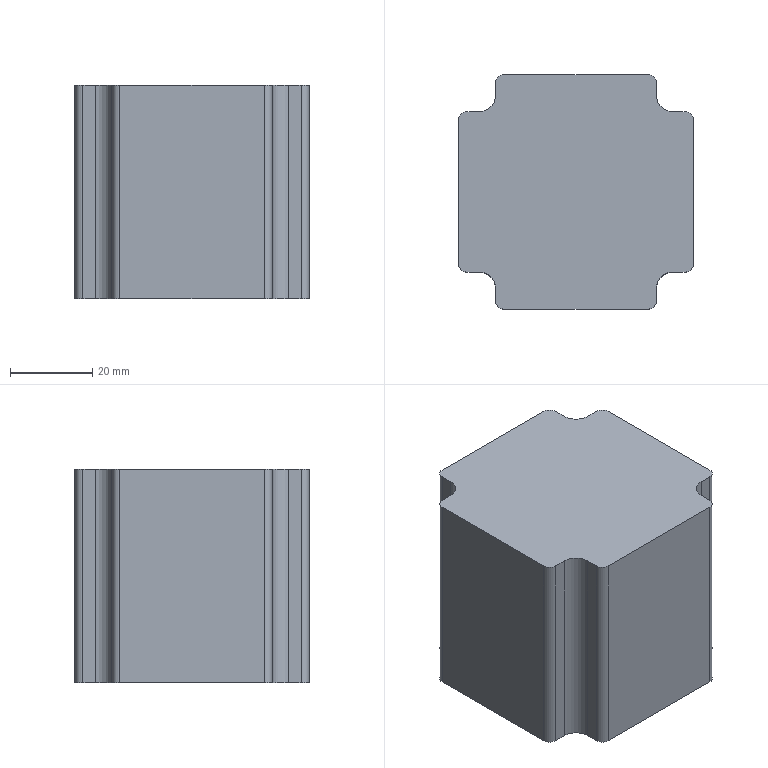Part | SolidWorks | features BaseBody 1 | 1 solid | 26 faces | box 57 x 57 x 52 mm | volume 152457 mm3 | plane 14 | cylinder 12 | commonest cylinder face diameters 4 x8 8 x4
STEP:
#1=CARTESIAN_POINT('',(19.5,26.5,0.));
#2=VERTEX_POINT('',#1);
#3=CARTESIAN_POINT('',(17.5,28.5,0.));
#4=VERTEX_POINT('',#3);
#5=CARTESIAN_POINT('',(17.5,26.5,0.));
#6=DIRECTION('',(0.,0.,1.));
#7=DIRECTION('',(-1.,0.,0.));
#8=AXIS2_PLACEMENT_3D('',#5,#6,#7);
#9=CIRCLE('',#8,2.);
#10=EDGE_CURVE('',#2,#4,#9,.T.);
#11=ORIENTED_EDGE('',*,*,#10,.F.);
#12=CARTESIAN_POINT('',(19.5,23.5,0.));
#13=VERTEX_POINT('',#12);
#14=CARTESIAN_POINT('',(19.5,26.5,0.));
#15=DIRECTION('',(0.,1.,0.));
#16=VECTOR('',#15,1000.);
#17=LINE('',#14,#16);
#18=EDGE_CURVE('',#13,#2,#17,.T.);
#19=ORIENTED_EDGE('',*,*,#18,.F.);
#20=CARTESIAN_POINT('',(23.5,19.5,0.));
#21=VERTEX_POINT('',#20);
#22=CARTESIAN_POINT('',(23.5,23.5,0.));
#23=DIRECTION('',(0.,0.,-1.));
#24=DIRECTION('',(1.,0.,0.));
#25=AXIS2_PLACEMENT_3D('',#22,#23,#24);
#26=CIRCLE('',#25,4.);
#27=EDGE_CURVE('',#21,#13,#26,.T.);
#28=ORIENTED_EDGE('',*,*,#27,.F.);
#29=CARTESIAN_POINT('',(26.5,19.5,0.));
#30=VERTEX_POINT('',#29);
#31=CARTESIAN_POINT('',(23.5,19.5,0.));
#32=DIRECTION('',(-1.,0.,0.));
#33=VECTOR('',#32,1000.);
#34=LINE('',#31,#33);
#35=EDGE_CURVE('',#30,#21,#34,.T.);
#36=ORIENTED_EDGE('',*,*,#35,.F.);
#37=CARTESIAN_POINT('',(28.5,17.5,0.));
#38=VERTEX_POINT('',#37);
#39=CARTESIAN_POINT('',(26.5,17.5,0.));
#40=DIRECTION('',(0.,0.,1.));
#41=DIRECTION('',(-1.,0.,0.));
#42=AXIS2_PLACEMENT_3D('',#39,#40,#41);
#43=CIRCLE('',#42,2.);
#44=EDGE_CURVE('',#38,#30,#43,.T.);
#45=ORIENTED_EDGE('',*,*,#44,.F.);
#46=CARTESIAN_POINT('',(28.5,-17.5,0.));
#47=VERTEX_POINT('',#46);
#48=CARTESIAN_POINT('',(28.5,17.5,0.));
#49=DIRECTION('',(0.,1.,0.));
#50=VECTOR('',#49,1000.);
#51=LINE('',#48,#50);
#52=EDGE_CURVE('',#47,#38,#51,.T.);
#53=ORIENTED_EDGE('',*,*,#52,.F.);
#54=CARTESIAN_POINT('',(26.5,-19.5,0.));
#55=VERTEX_POINT('',#54);
#56=CARTESIAN_POINT('',(26.5,-17.5,0.));
#57=DIRECTION('',(0.,0.,1.));
#58=DIRECTION('',(-1.,0.,0.));
#59=AXIS2_PLACEMENT_3D('',#56,#57,#58);
#60=CIRCLE('',#59,2.);
#61=EDGE_CURVE('',#55,#47,#60,.T.);
#62=ORIENTED_EDGE('',*,*,#61,.F.);
#63=CARTESIAN_POINT('',(23.5,-19.5,0.));
#64=VERTEX_POINT('',#63);
#65=CARTESIAN_POINT('',(26.5,-19.5,0.));
#66=DIRECTION('',(1.,0.,0.));
#67=VECTOR('',#66,1000.);
#68=LINE('',#65,#67);
#69=EDGE_CURVE('',#64,#55,#68,.T.);
#70=ORIENTED_EDGE('',*,*,#69,.F.);
#71=CARTESIAN_POINT('',(19.5,-23.5,0.));
#72=VERTEX_POINT('',#71);
#73=CARTESIAN_POINT('',(23.5,-23.5,0.));
#74=DIRECTION('',(0.,0.,-1.));
#75=DIRECTION('',(-1.,0.,0.));
#76=AXIS2_PLACEMENT_3D('',#73,#74,#75);
#77=CIRCLE('',#76,4.);
#78=EDGE_CURVE('',#72,#64,#77,.T.);
#79=ORIENTED_EDGE('',*,*,#78,.F.);
#80=CARTESIAN_POINT('',(19.5,-26.5,0.));
#81=VERTEX_POINT('',#80);
#82=CARTESIAN_POINT('',(19.5,-23.5,0.));
#83=DIRECTION('',(0.,1.,0.));
#84=VECTOR('',#83,1000.);
#85=LINE('',#82,#84);
#86=EDGE_CURVE('',#81,#72,#85,.T.);
#87=ORIENTED_EDGE('',*,*,#86,.F.);
#88=CARTESIAN_POINT('',(17.5,-28.5,0.));
#89=VERTEX_POINT('',#88);
#90=CARTESIAN_POINT('',(17.5,-26.5,0.));
#91=DIRECTION('',(0.,0.,1.));
#92=DIRECTION('',(-1.,0.,0.));
#93=AXIS2_PLACEMENT_3D('',#90,#91,#92);
#94=CIRCLE('',#93,2.);
#95=EDGE_CURVE('',#89,#81,#94,.T.);
#96=ORIENTED_EDGE('',*,*,#95,.F.);
#97=CARTESIAN_POINT('',(-17.5,-28.5,0.));
#98=VERTEX_POINT('',#97);
#99=CARTESIAN_POINT('',(17.5,-28.5,0.));
#100=DIRECTION('',(1.,0.,0.));
#101=VECTOR('',#100,1000.);
#102=LINE('',#99,#101);
#103=EDGE_CURVE('',#98,#89,#102,.T.);
#104=ORIENTED_EDGE('',*,*,#103,.F.);
#105=CARTESIAN_POINT('',(-19.5,-26.5,0.));
#106=VERTEX_POINT('',#105);
#107=CARTESIAN_POINT('',(-17.5,-26.5,0.));
#108=DIRECTION('',(0.,0.,1.));
#109=DIRECTION('',(-1.,0.,0.));
#110=AXIS2_PLACEMENT_3D('',#107,#108,#109);
#111=CIRCLE('',#110,2.);
#112=EDGE_CURVE('',#106,#98,#111,.T.);
#113=ORIENTED_EDGE('',*,*,#112,.F.);
#114=CARTESIAN_POINT('',(-19.5,-23.5,0.));
#115=VERTEX_POINT('',#114);
#116=CARTESIAN_POINT('',(-19.5,-26.5,0.));
#117=DIRECTION('',(0.,-1.,0.));
#118=VECTOR('',#117,1000.);
#119=LINE('',#116,#118);
#120=EDGE_CURVE('',#115,#106,#119,.T.);
#121=ORIENTED_EDGE('',*,*,#120,.F.);
#122=CARTESIAN_POINT('',(-23.5,-19.5,0.));
#123=VERTEX_POINT('',#122);
#124=CARTESIAN_POINT('',(-23.5,-23.5,0.));
#125=DIRECTION('',(0.,0.,-1.));
#126=DIRECTION('',(1.,0.,0.));
#127=AXIS2_PLACEMENT_3D('',#124,#125,#126);
#128=CIRCLE('',#127,4.);
#129=EDGE_CURVE('',#123,#115,#128,.T.);
#130=ORIENTED_EDGE('',*,*,#129,.F.);
#131=CARTESIAN_POINT('',(-26.5,-19.5,0.));
#132=VERTEX_POINT('',#131);
#133=CARTESIAN_POINT('',(-23.5,-19.5,0.));
#134=DIRECTION('',(1.,0.,0.));
#135=VECTOR('',#134,1000.);
#136=LINE('',#133,#135);
#137=EDGE_CURVE('',#132,#123,#136,.T.);
#138=ORIENTED_EDGE('',*,*,#137,.F.);
#139=CARTESIAN_POINT('',(-28.5,-17.5,0.));
#140=VERTEX_POINT('',#139);
#141=CARTESIAN_POINT('',(-26.5,-17.5,0.));
#142=DIRECTION('',(0.,0.,1.));
#143=DIRECTION('',(-1.,0.,0.));
#144=AXIS2_PLACEMENT_3D('',#141,#142,#143);
#145=CIRCLE('',#144,2.);
#146=EDGE_CURVE('',#140,#132,#145,.T.);
#147=ORIENTED_EDGE('',*,*,#146,.F.);
#148=CARTESIAN_POINT('',(-28.5,17.5,0.));
#149=VERTEX_POINT('',#148);
#150=CARTESIAN_POINT('',(-28.5,-17.5,0.));
#151=DIRECTION('',(0.,-1.,0.));
#152=VECTOR('',#151,1000.);
#153=LINE('',#150,#152);
#154=EDGE_CURVE('',#149,#140,#153,.T.);
#155=ORIENTED_EDGE('',*,*,#154,.F.);
#156=CARTESIAN_POINT('',(-26.5,19.5,0.));
#157=VERTEX_POINT('',#156);
#158=CARTESIAN_POINT('',(-26.5,17.5,0.));
#159=DIRECTION('',(0.,0.,1.));
#160=DIRECTION('',(-1.,0.,0.));
#161=AXIS2_PLACEMENT_3D('',#158,#159,#160);
#162=CIRCLE('',#161,2.);
#163=EDGE_CURVE('',#157,#149,#162,.T.);
#164=ORIENTED_EDGE('',*,*,#163,.F.);
#165=CARTESIAN_POINT('',(-23.5,19.5,0.));
#166=VERTEX_POINT('',#165);
#167=CARTESIAN_POINT('',(-26.5,19.5,0.));
#168=DIRECTION('',(-1.,0.,0.));
#169=VECTOR('',#168,1000.);
#170=LINE('',#167,#169);
#171=EDGE_CURVE('',#166,#157,#170,.T.);
#172=ORIENTED_EDGE('',*,*,#171,.F.);
#173=CARTESIAN_POINT('',(-19.5,23.5,0.));
#174=VERTEX_POINT('',#173);
#175=CARTESIAN_POINT('',(-23.5,23.5,0.));
#176=DIRECTION('',(0.,0.,-1.));
#177=DIRECTION('',(1.,0.,0.));
#178=AXIS2_PLACEMENT_3D('',#175,#176,#177);
#179=CIRCLE('',#178,4.);
#180=EDGE_CURVE('',#174,#166,#179,.T.);
#181=ORIENTED_EDGE('',*,*,#180,.F.);
#182=CARTESIAN_POINT('',(-19.5,26.5,0.));
#183=VERTEX_POINT('',#182);
#184=CARTESIAN_POINT('',(-19.5,23.5,0.));
#185=DIRECTION('',(0.,-1.,0.));
#186=VECTOR('',#185,1000.);
#187=LINE('',#184,#186);
#188=EDGE_CURVE('',#183,#174,#187,.T.);
#189=ORIENTED_EDGE('',*,*,#188,.F.);
#190=CARTESIAN_POINT('',(-17.5,28.5,0.));
#191=VERTEX_POINT('',#190);
#192=CARTESIAN_POINT('',(-17.5,26.5,0.));
#193=DIRECTION('',(0.,0.,1.));
#194=DIRECTION('',(-1.,0.,0.));
#195=AXIS2_PLACEMENT_3D('',#192,#193,#194);
#196=CIRCLE('',#195,2.);
#197=EDGE_CURVE('',#191,#183,#196,.T.);
#198=ORIENTED_EDGE('',*,*,#197,.F.);
#199=CARTESIAN_POINT('',(-17.5,28.5,0.));
#200=DIRECTION('',(-1.,0.,0.));
#201=VECTOR('',#200,1000.);
#202=LINE('',#199,#201);
#203=EDGE_CURVE('',#4,#191,#202,.T.);
#204=ORIENTED_EDGE('',*,*,#203,.F.);
#205=EDGE_LOOP('',(#11,#19,#28,#36,#45,#53,#62,#70,#79,#87,#96,#104,#113,#121,#130,#138,#147,#155,#164,#172,#181,#189,#198,#204));
#206=FACE_OUTER_BOUND('',#205,.T.);
#207=CARTESIAN_POINT('',(17.5,26.5,0.));
#208=DIRECTION('',(0.,0.,-1.));
#209=DIRECTION('',(0.,-1.,0.));
#210=AXIS2_PLACEMENT_3D('',#207,#208,#209);
#211=PLANE('',#210);
#212=ADVANCED_FACE('',(#206),#211,.T.);
#213=CARTESIAN_POINT('',(19.5,26.5,52.));
#214=VERTEX_POINT('',#213);
#215=CARTESIAN_POINT('',(17.5,28.5,52.));
#216=VERTEX_POINT('',#215);
#217=CARTESIAN_POINT('',(17.5,26.5,52.));
#218=DIRECTION('',(0.,0.,1.));
#219=DIRECTION('',(-1.,0.,0.));
#220=AXIS2_PLACEMENT_3D('',#217,#218,#219);
#221=CIRCLE('',#220,2.);
#222=EDGE_CURVE('',#214,#216,#221,.T.);
#223=ORIENTED_EDGE('',*,*,#222,.T.);
#224=CARTESIAN_POINT('',(-17.5,28.5,52.));
#225=VERTEX_POINT('',#224);
#226=CARTESIAN_POINT('',(-17.5,28.5,52.));
#227=DIRECTION('',(-1.,0.,0.));
#228=VECTOR('',#227,1000.);
#229=LINE('',#226,#228);
#230=EDGE_CURVE('',#216,#225,#229,.T.);
#231=ORIENTED_EDGE('',*,*,#230,.T.);
#232=CARTESIAN_POINT('',(-19.5,26.5,52.));
#233=VERTEX_POINT('',#232);
#234=CARTESIAN_POINT('',(-17.5,26.5,52.));
#235=DIRECTION('',(0.,0.,1.));
#236=DIRECTION('',(-1.,0.,0.));
#237=AXIS2_PLACEMENT_3D('',#234,#235,#236);
#238=CIRCLE('',#237,2.);
#239=EDGE_CURVE('',#225,#233,#238,.T.);
#240=ORIENTED_EDGE('',*,*,#239,.T.);
#241=CARTESIAN_POINT('',(-19.5,23.5,52.));
#242=VERTEX_POINT('',#241);
#243=CARTESIAN_POINT('',(-19.5,23.5,52.));
#244=DIRECTION('',(0.,-1.,0.));
#245=VECTOR('',#244,1000.);
#246=LINE('',#243,#245);
#247=EDGE_CURVE('',#233,#242,#246,.T.);
#248=ORIENTED_EDGE('',*,*,#247,.T.);
#249=CARTESIAN_POINT('',(-23.5,19.5,52.));
#250=VERTEX_POINT('',#249);
#251=CARTESIAN_POINT('',(-23.5,23.5,52.));
#252=DIRECTION('',(0.,0.,-1.));
#253=DIRECTION('',(1.,0.,0.));
#254=AXIS2_PLACEMENT_3D('',#251,#252,#253);
#255=CIRCLE('',#254,4.);
#256=EDGE_CURVE('',#242,#250,#255,.T.);
#257=ORIENTED_EDGE('',*,*,#256,.T.);
#258=CARTESIAN_POINT('',(-26.5,19.5,52.));
#259=VERTEX_POINT('',#258);
#260=CARTESIAN_POINT('',(-26.5,19.5,52.));
#261=DIRECTION('',(-1.,0.,0.));
#262=VECTOR('',#261,1000.);
#263=LINE('',#260,#262);
#264=EDGE_CURVE('',#250,#259,#263,.T.);
#265=ORIENTED_EDGE('',*,*,#264,.T.);
#266=CARTESIAN_POINT('',(-28.5,17.5,52.));
#267=VERTEX_POINT('',#266);
#268=CARTESIAN_POINT('',(-26.5,17.5,52.));
#269=DIRECTION('',(0.,0.,1.));
#270=DIRECTION('',(-1.,0.,0.));
#271=AXIS2_PLACEMENT_3D('',#268,#269,#270);
#272=CIRCLE('',#271,2.);
#273=EDGE_CURVE('',#259,#267,#272,.T.);
#274=ORIENTED_EDGE('',*,*,#273,.T.);
#275=CARTESIAN_POINT('',(-28.5,-17.5,52.));
#276=VERTEX_POINT('',#275);
#277=CARTESIAN_POINT('',(-28.5,-17.5,52.));
#278=DIRECTION('',(0.,-1.,0.));
#279=VECTOR('',#278,1000.);
#280=LINE('',#277,#279);
#281=EDGE_CURVE('',#267,#276,#280,.T.);
#282=ORIENTED_EDGE('',*,*,#281,.T.);
#283=CARTESIAN_POINT('',(-26.5,-19.5,52.));
#284=VERTEX_POINT('',#283);
#285=CARTESIAN_POINT('',(-26.5,-17.5,52.));
#286=DIRECTION('',(0.,0.,1.));
#287=DIRECTION('',(-1.,0.,0.));
#288=AXIS2_PLACEMENT_3D('',#285,#286,#287);
#289=CIRCLE('',#288,2.);
#290=EDGE_CURVE('',#276,#284,#289,.T.);
#291=ORIENTED_EDGE('',*,*,#290,.T.);
#292=CARTESIAN_POINT('',(-23.5,-19.5,52.));
#293=VERTEX_POINT('',#292);
#294=CARTESIAN_POINT('',(-23.5,-19.5,52.));
#295=DIRECTION('',(1.,0.,0.));
#296=VECTOR('',#295,1000.);
#297=LINE('',#294,#296);
#298=EDGE_CURVE('',#284,#293,#297,.T.);
#299=ORIENTED_EDGE('',*,*,#298,.T.);
#300=CARTESIAN_POINT('',(-19.5,-23.5,52.));
#301=VERTEX_POINT('',#300);
#302=CARTESIAN_POINT('',(-23.5,-23.5,52.));
#303=DIRECTION('',(0.,0.,-1.));
#304=DIRECTION('',(1.,0.,0.));
#305=AXIS2_PLACEMENT_3D('',#302,#303,#304);
#306=CIRCLE('',#305,4.);
#307=EDGE_CURVE('',#293,#301,#306,.T.);
#308=ORIENTED_EDGE('',*,*,#307,.T.);
#309=CARTESIAN_POINT('',(-19.5,-26.5,52.));
#310=VERTEX_POINT('',#309);
#311=CARTESIAN_POINT('',(-19.5,-26.5,52.));
#312=DIRECTION('',(0.,-1.,0.));
#313=VECTOR('',#312,1000.);
#314=LINE('',#311,#313);
#315=EDGE_CURVE('',#301,#310,#314,.T.);
#316=ORIENTED_EDGE('',*,*,#315,.T.);
#317=CARTESIAN_POINT('',(-17.5,-28.5,52.));
#318=VERTEX_POINT('',#317);
#319=CARTESIAN_POINT('',(-17.5,-26.5,52.));
#320=DIRECTION('',(0.,0.,1.));
#321=DIRECTION('',(-1.,0.,0.));
#322=AXIS2_PLACEMENT_3D('',#319,#320,#321);
#323=CIRCLE('',#322,2.);
#324=EDGE_CURVE('',#310,#318,#323,.T.);
#325=ORIENTED_EDGE('',*,*,#324,.T.);
#326=CARTESIAN_POINT('',(17.5,-28.5,52.));
#327=VERTEX_POINT('',#326);
#328=CARTESIAN_POINT('',(17.5,-28.5,52.));
#329=DIRECTION('',(1.,0.,0.));
#330=VECTOR('',#329,1000.);
#331=LINE('',#328,#330);
#332=EDGE_CURVE('',#318,#327,#331,.T.);
#333=ORIENTED_EDGE('',*,*,#332,.T.);
#334=CARTESIAN_POINT('',(19.5,-26.5,52.));
#335=VERTEX_POINT('',#334);
#336=CARTESIAN_POINT('',(17.5,-26.5,52.));
#337=DIRECTION('',(0.,0.,1.));
#338=DIRECTION('',(-1.,0.,0.));
#339=AXIS2_PLACEMENT_3D('',#336,#337,#338);
#340=CIRCLE('',#339,2.);
#341=EDGE_CURVE('',#327,#335,#340,.T.);
#342=ORIENTED_EDGE('',*,*,#341,.T.);
#343=CARTESIAN_POINT('',(19.5,-23.5,52.));
#344=VERTEX_POINT('',#343);
#345=CARTESIAN_POINT('',(19.5,-23.5,52.));
#346=DIRECTION('',(0.,1.,0.));
#347=VECTOR('',#346,1000.);
#348=LINE('',#345,#347);
#349=EDGE_CURVE('',#335,#344,#348,.T.);
#350=ORIENTED_EDGE('',*,*,#349,.T.);
#351=CARTESIAN_POINT('',(23.5,-19.5,52.));
#352=VERTEX_POINT('',#351);
#353=CARTESIAN_POINT('',(23.5,-23.5,52.));
#354=DIRECTION('',(0.,0.,-1.));
#355=DIRECTION('',(-1.,0.,0.));
#356=AXIS2_PLACEMENT_3D('',#353,#354,#355);
#357=CIRCLE('',#356,4.);
#358=EDGE_CURVE('',#344,#352,#357,.T.);
#359=ORIENTED_EDGE('',*,*,#358,.T.);
#360=CARTESIAN_POINT('',(26.5,-19.5,52.));
#361=VERTEX_POINT('',#360);
#362=CARTESIAN_POINT('',(26.5,-19.5,52.));
#363=DIRECTION('',(1.,0.,0.));
#364=VECTOR('',#363,1000.);
#365=LINE('',#362,#364);
#366=EDGE_CURVE('',#352,#361,#365,.T.);
#367=ORIENTED_EDGE('',*,*,#366,.T.);
#368=CARTESIAN_POINT('',(28.5,-17.5,52.));
#369=VERTEX_POINT('',#368);
#370=CARTESIAN_POINT('',(26.5,-17.5,52.));
#371=DIRECTION('',(0.,0.,1.));
#372=DIRECTION('',(-1.,0.,0.));
#373=AXIS2_PLACEMENT_3D('',#370,#371,#372);
#374=CIRCLE('',#373,2.);
#375=EDGE_CURVE('',#361,#369,#374,.T.);
#376=ORIENTED_EDGE('',*,*,#375,.T.);
#377=CARTESIAN_POINT('',(28.5,17.5,52.));
#378=VERTEX_POINT('',#377);
#379=CARTESIAN_POINT('',(28.5,17.5,52.));
#380=DIRECTION('',(0.,1.,0.));
#381=VECTOR('',#380,1000.);
#382=LINE('',#379,#381);
#383=EDGE_CURVE('',#369,#378,#382,.T.);
#384=ORIENTED_EDGE('',*,*,#383,.T.);
#385=CARTESIAN_POINT('',(26.5,19.5,52.));
#386=VERTEX_POINT('',#385);
#387=CARTESIAN_POINT('',(26.5,17.5,52.));
#388=DIRECTION('',(0.,0.,1.));
#389=DIRECTION('',(-1.,0.,0.));
#390=AXIS2_PLACEMENT_3D('',#387,#388,#389);
#391=CIRCLE('',#390,2.);
#392=EDGE_CURVE('',#378,#386,#391,.T.);
#393=ORIENTED_EDGE('',*,*,#392,.T.);
#394=CARTESIAN_POINT('',(23.5,19.5,52.));
#395=VERTEX_POINT('',#394);
#396=CARTESIAN_POINT('',(23.5,19.5,52.));
#397=DIRECTION('',(-1.,0.,0.));
#398=VECTOR('',#397,1000.);
#399=LINE('',#396,#398);
#400=EDGE_CURVE('',#386,#395,#399,.T.);
#401=ORIENTED_EDGE('',*,*,#400,.T.);
#402=CARTESIAN_POINT('',(19.5,23.5,52.));
#403=VERTEX_POINT('',#402);
#404=CARTESIAN_POINT('',(23.5,23.5,52.));
#405=DIRECTION('',(0.,0.,-1.));
#406=DIRECTION('',(1.,0.,0.));
#407=AXIS2_PLACEMENT_3D('',#404,#405,#406);
#408=CIRCLE('',#407,4.);
#409=EDGE_CURVE('',#395,#403,#408,.T.);
#410=ORIENTED_EDGE('',*,*,#409,.T.);
#411=CARTESIAN_POINT('',(19.5,26.5,52.));
#412=DIRECTION('',(0.,1.,0.));
#413=VECTOR('',#412,1000.);
#414=LINE('',#411,#413);
#415=EDGE_CURVE('',#403,#214,#414,.T.);
#416=ORIENTED_EDGE('',*,*,#415,.T.);
#417=EDGE_LOOP('',(#223,#231,#240,#248,#257,#265,#274,#282,#291,#299,#308,#316,#325,#333,#342,#350,#359,#367,#376,#384,#393,#401,#410,#416));
#418=FACE_OUTER_BOUND('',#417,.T.);
#419=CARTESIAN_POINT('',(17.5,26.5,52.));
#420=DIRECTION('',(0.,0.,-1.));
#421=DIRECTION('',(0.,-1.,0.));
#422=AXIS2_PLACEMENT_3D('',#419,#420,#421);
#423=PLANE('',#422);
#424=ADVANCED_FACE('',(#418),#423,.F.);
#425=ORIENTED_EDGE('',*,*,#18,.T.);
#426=CARTESIAN_POINT('',(19.5,26.5,54.));
#427=DIRECTION('',(0.,0.,-1.));
#428=VECTOR('',#427,1000.);
#429=LINE('',#426,#428);
#430=EDGE_CURVE('',#214,#2,#429,.T.);
#431=ORIENTED_EDGE('',*,*,#430,.F.);
#432=ORIENTED_EDGE('',*,*,#415,.F.);
#433=CARTESIAN_POINT('',(19.5,23.5,54.));
#434=DIRECTION('',(0.,0.,-1.));
#435=VECTOR('',#434,1000.);
#436=LINE('',#433,#435);
#437=EDGE_CURVE('',#403,#13,#436,.T.);
#438=ORIENTED_EDGE('',*,*,#437,.T.);
#439=EDGE_LOOP('',(#425,#431,#432,#438));
#440=FACE_OUTER_BOUND('',#439,.T.);
#441=CARTESIAN_POINT('',(19.5,26.5,54.));
#442=DIRECTION('',(-1.,0.,0.));
#443=DIRECTION('',(0.,0.,1.));
#444=AXIS2_PLACEMENT_3D('',#441,#442,#443);
#445=PLANE('',#444);
#446=ADVANCED_FACE('',(#440),#445,.F.);
#447=ORIENTED_EDGE('',*,*,#27,.T.);
#448=ORIENTED_EDGE('',*,*,#437,.F.);
#449=ORIENTED_EDGE('',*,*,#409,.F.);
#450=CARTESIAN_POINT('',(23.5,19.5,54.));
#451=DIRECTION('',(0.,0.,-1.));
#452=VECTOR('',#451,1000.);
#453=LINE('',#450,#452);
#454=EDGE_CURVE('',#395,#21,#453,.T.);
#455=ORIENTED_EDGE('',*,*,#454,.T.);
#456=EDGE_LOOP('',(#447,#448,#449,#455));
#457=FACE_OUTER_BOUND('',#456,.T.);
#458=CARTESIAN_POINT('',(23.5,23.5,54.));
#459=DIRECTION('',(0.,0.,-1.));
#460=DIRECTION('',(-1.,0.,0.));
#461=AXIS2_PLACEMENT_3D('',#458,#459,#460);
#462=CYLINDRICAL_SURFACE('',#461,4.);
#463=ADVANCED_FACE('',(#457),#462,.F.);
#464=ORIENTED_EDGE('',*,*,#35,.T.);
#465=ORIENTED_EDGE('',*,*,#454,.F.);
#466=ORIENTED_EDGE('',*,*,#400,.F.);
#467=CARTESIAN_POINT('',(26.5,19.5,54.));
#468=DIRECTION('',(0.,0.,-1.));
#469=VECTOR('',#468,1000.);
#470=LINE('',#467,#469);
#471=EDGE_CURVE('',#386,#30,#470,.T.);
#472=ORIENTED_EDGE('',*,*,#471,.T.);
#473=EDGE_LOOP('',(#464,#465,#466,#472));
#474=FACE_OUTER_BOUND('',#473,.T.);
#475=CARTESIAN_POINT('',(23.5,19.5,54.));
#476=DIRECTION('',(0.,-1.,0.));
#477=DIRECTION('',(0.,0.,-1.));
#478=AXIS2_PLACEMENT_3D('',#475,#476,#477);
#479=PLANE('',#478);
#480=ADVANCED_FACE('',(#474),#479,.F.);
#481=ORIENTED_EDGE('',*,*,#44,.T.);
#482=ORIENTED_EDGE('',*,*,#471,.F.);
#483=ORIENTED_EDGE('',*,*,#392,.F.);
#484=CARTESIAN_POINT('',(28.5,17.5,54.));
#485=DIRECTION('',(0.,0.,-1.));
#486=VECTOR('',#485,1000.);
#487=LINE('',#484,#486);
#488=EDGE_CURVE('',#378,#38,#487,.T.);
#489=ORIENTED_EDGE('',*,*,#488,.T.);
#490=EDGE_LOOP('',(#481,#482,#483,#489));
#491=FACE_OUTER_BOUND('',#490,.T.);
#492=CARTESIAN_POINT('',(26.5,17.5,54.));
#493=DIRECTION('',(0.,0.,-1.));
#494=DIRECTION('',(-1.,0.,0.));
#495=AXIS2_PLACEMENT_3D('',#492,#493,#494);
#496=CYLINDRICAL_SURFACE('',#495,2.);
#497=ADVANCED_FACE('',(#491),#496,.T.);
#498=ORIENTED_EDGE('',*,*,#52,.T.);
#499=ORIENTED_EDGE('',*,*,#488,.F.);
#500=ORIENTED_EDGE('',*,*,#383,.F.);
#501=CARTESIAN_POINT('',(28.5,-17.5,54.));
#502=DIRECTION('',(0.,0.,-1.));
#503=VECTOR('',#502,1000.);
#504=LINE('',#501,#503);
#505=EDGE_CURVE('',#369,#47,#504,.T.);
#506=ORIENTED_EDGE('',*,*,#505,.T.);
#507=EDGE_LOOP('',(#498,#499,#500,#506));
#508=FACE_OUTER_BOUND('',#507,.T.);
#509=CARTESIAN_POINT('',(28.5,17.5,54.));
#510=DIRECTION('',(-1.,0.,0.));
#511=DIRECTION('',(0.,1.,0.));
#512=AXIS2_PLACEMENT_3D('',#509,#510,#511);
#513=PLANE('',#512);
#514=ADVANCED_FACE('',(#508),#513,.F.);
#515=ORIENTED_EDGE('',*,*,#61,.T.);
#516=ORIENTED_EDGE('',*,*,#505,.F.);
#517=ORIENTED_EDGE('',*,*,#375,.F.);
#518=CARTESIAN_POINT('',(26.5,-19.5,54.));
#519=DIRECTION('',(0.,0.,-1.));
#520=VECTOR('',#519,1000.);
#521=LINE('',#518,#520);
#522=EDGE_CURVE('',#361,#55,#521,.T.);
#523=ORIENTED_EDGE('',*,*,#522,.T.);
#524=EDGE_LOOP('',(#515,#516,#517,#523));
#525=FACE_OUTER_BOUND('',#524,.T.);
#526=CARTESIAN_POINT('',(26.5,-17.5,54.));
#527=DIRECTION('',(0.,0.,-1.));
#528=DIRECTION('',(-1.,0.,0.));
#529=AXIS2_PLACEMENT_3D('',#526,#527,#528);
#530=CYLINDRICAL_SURFACE('',#529,2.);
#531=ADVANCED_FACE('',(#525),#530,.T.);
#532=ORIENTED_EDGE('',*,*,#69,.T.);
#533=ORIENTED_EDGE('',*,*,#522,.F.);
#534=ORIENTED_EDGE('',*,*,#366,.F.);
#535=CARTESIAN_POINT('',(23.5,-19.5,54.));
#536=DIRECTION('',(0.,0.,-1.));
#537=VECTOR('',#536,1000.);
#538=LINE('',#535,#537);
#539=EDGE_CURVE('',#352,#64,#538,.T.);
#540=ORIENTED_EDGE('',*,*,#539,.T.);
#541=EDGE_LOOP('',(#532,#533,#534,#540));
#542=FACE_OUTER_BOUND('',#541,.T.);
#543=CARTESIAN_POINT('',(26.5,-19.5,54.));
#544=DIRECTION('',(0.,1.,0.));
#545=DIRECTION('',(1.,0.,0.));
#546=AXIS2_PLACEMENT_3D('',#543,#544,#545);
#547=PLANE('',#546);
#548=ADVANCED_FACE('',(#542),#547,.F.);
#549=ORIENTED_EDGE('',*,*,#78,.T.);
#550=ORIENTED_EDGE('',*,*,#539,.F.);
#551=ORIENTED_EDGE('',*,*,#358,.F.);
#552=CARTESIAN_POINT('',(19.5,-23.5,54.));
#553=DIRECTION('',(0.,0.,-1.));
#554=VECTOR('',#553,1000.);
#555=LINE('',#552,#554);
#556=EDGE_CURVE('',#344,#72,#555,.T.);
#557=ORIENTED_EDGE('',*,*,#556,.T.);
#558=EDGE_LOOP('',(#549,#550,#551,#557));
#559=FACE_OUTER_BOUND('',#558,.T.);
#560=CARTESIAN_POINT('',(23.5,-23.5,54.));
#561=DIRECTION('',(0.,0.,-1.));
#562=DIRECTION('',(-1.,0.,0.));
#563=AXIS2_PLACEMENT_3D('',#560,#561,#562);
#564=CYLINDRICAL_SURFACE('',#563,4.);
#565=ADVANCED_FACE('',(#559),#564,.F.);
#566=ORIENTED_EDGE('',*,*,#86,.T.);
#567=ORIENTED_EDGE('',*,*,#556,.F.);
#568=ORIENTED_EDGE('',*,*,#349,.F.);
#569=CARTESIAN_POINT('',(19.5,-26.5,54.));
#570=DIRECTION('',(0.,0.,-1.));
#571=VECTOR('',#570,1000.);
#572=LINE('',#569,#571);
#573=EDGE_CURVE('',#335,#81,#572,.T.);
#574=ORIENTED_EDGE('',*,*,#573,.T.);
#575=EDGE_LOOP('',(#566,#567,#568,#574));
#576=FACE_OUTER_BOUND('',#575,.T.);
#577=CARTESIAN_POINT('',(19.5,-23.5,54.));
#578=DIRECTION('',(-1.,0.,0.));
#579=DIRECTION('',(0.,0.,1.));
#580=AXIS2_PLACEMENT_3D('',#577,#578,#579);
#581=PLANE('',#580);
#582=ADVANCED_FACE('',(#576),#581,.F.);
#583=ORIENTED_EDGE('',*,*,#95,.T.);
#584=ORIENTED_EDGE('',*,*,#573,.F.);
#585=ORIENTED_EDGE('',*,*,#341,.F.);
#586=CARTESIAN_POINT('',(17.5,-28.5,54.));
#587=DIRECTION('',(0.,0.,-1.));
#588=VECTOR('',#587,1000.);
#589=LINE('',#586,#588);
#590=EDGE_CURVE('',#327,#89,#589,.T.);
#591=ORIENTED_EDGE('',*,*,#590,.T.);
#592=EDGE_LOOP('',(#583,#584,#585,#591));
#593=FACE_OUTER_BOUND('',#592,.T.);
#594=CARTESIAN_POINT('',(17.5,-26.5,54.));
#595=DIRECTION('',(0.,0.,-1.));
#596=DIRECTION('',(-1.,0.,0.));
#597=AXIS2_PLACEMENT_3D('',#594,#595,#596);
#598=CYLINDRICAL_SURFACE('',#597,2.);
#599=ADVANCED_FACE('',(#593),#598,.T.);
#600=ORIENTED_EDGE('',*,*,#103,.T.);
#601=ORIENTED_EDGE('',*,*,#590,.F.);
#602=ORIENTED_EDGE('',*,*,#332,.F.);
#603=CARTESIAN_POINT('',(-17.5,-28.5,54.));
#604=DIRECTION('',(0.,0.,-1.));
#605=VECTOR('',#604,1000.);
#606=LINE('',#603,#605);
#607=EDGE_CURVE('',#318,#98,#606,.T.);
#608=ORIENTED_EDGE('',*,*,#607,.T.);
#609=EDGE_LOOP('',(#600,#601,#602,#608));
#610=FACE_OUTER_BOUND('',#609,.T.);
#611=CARTESIAN_POINT('',(17.5,-28.5,54.));
#612=DIRECTION('',(0.,1.,0.));
#613=DIRECTION('',(1.,0.,0.));
#614=AXIS2_PLACEMENT_3D('',#611,#612,#613);
#615=PLANE('',#614);
#616=ADVANCED_FACE('',(#610),#615,.F.);
#617=ORIENTED_EDGE('',*,*,#112,.T.);
#618=ORIENTED_EDGE('',*,*,#607,.F.);
#619=ORIENTED_EDGE('',*,*,#324,.F.);
#620=CARTESIAN_POINT('',(-19.5,-26.5,54.));
#621=DIRECTION('',(0.,0.,-1.));
#622=VECTOR('',#621,1000.);
#623=LINE('',#620,#622);
#624=EDGE_CURVE('',#310,#106,#623,.T.);
#625=ORIENTED_EDGE('',*,*,#624,.T.);
#626=EDGE_LOOP('',(#617,#618,#619,#625));
#627=FACE_OUTER_BOUND('',#626,.T.);
#628=CARTESIAN_POINT('',(-17.5,-26.5,54.));
#629=DIRECTION('',(0.,0.,-1.));
#630=DIRECTION('',(-1.,0.,0.));
#631=AXIS2_PLACEMENT_3D('',#628,#629,#630);
#632=CYLINDRICAL_SURFACE('',#631,2.);
#633=ADVANCED_FACE('',(#627),#632,.T.);
#634=ORIENTED_EDGE('',*,*,#120,.T.);
#635=ORIENTED_EDGE('',*,*,#624,.F.);
#636=ORIENTED_EDGE('',*,*,#315,.F.);
#637=CARTESIAN_POINT('',(-19.5,-23.5,54.));
#638=DIRECTION('',(0.,0.,-1.));
#639=VECTOR('',#638,1000.);
#640=LINE('',#637,#639);
#641=EDGE_CURVE('',#301,#115,#640,.T.);
#642=ORIENTED_EDGE('',*,*,#641,.T.);
#643=EDGE_LOOP('',(#634,#635,#636,#642));
#644=FACE_OUTER_BOUND('',#643,.T.);
#645=CARTESIAN_POINT('',(-19.5,-26.5,54.));
#646=DIRECTION('',(1.,0.,0.));
#647=DIRECTION('',(0.,1.,0.));
#648=AXIS2_PLACEMENT_3D('',#645,#646,#647);
#649=PLANE('',#648);
#650=ADVANCED_FACE('',(#644),#649,.F.);
#651=ORIENTED_EDGE('',*,*,#129,.T.);
#652=ORIENTED_EDGE('',*,*,#641,.F.);
#653=ORIENTED_EDGE('',*,*,#307,.F.);
#654=CARTESIAN_POINT('',(-23.5,-19.5,54.));
#655=DIRECTION('',(0.,0.,-1.));
#656=VECTOR('',#655,1000.);
#657=LINE('',#654,#656);
#658=EDGE_CURVE('',#293,#123,#657,.T.);
#659=ORIENTED_EDGE('',*,*,#658,.T.);
#660=EDGE_LOOP('',(#651,#652,#653,#659));
#661=FACE_OUTER_BOUND('',#660,.T.);
#662=CARTESIAN_POINT('',(-23.5,-23.5,54.));
#663=DIRECTION('',(0.,0.,-1.));
#664=DIRECTION('',(-1.,0.,0.));
#665=AXIS2_PLACEMENT_3D('',#662,#663,#664);
#666=CYLINDRICAL_SURFACE('',#665,4.);
#667=ADVANCED_FACE('',(#661),#666,.F.);
#668=ORIENTED_EDGE('',*,*,#137,.T.);
#669=ORIENTED_EDGE('',*,*,#658,.F.);
#670=ORIENTED_EDGE('',*,*,#298,.F.);
#671=CARTESIAN_POINT('',(-26.5,-19.5,54.));
#672=DIRECTION('',(0.,0.,-1.));
#673=VECTOR('',#672,1000.);
#674=LINE('',#671,#673);
#675=EDGE_CURVE('',#284,#132,#674,.T.);
#676=ORIENTED_EDGE('',*,*,#675,.T.);
#677=EDGE_LOOP('',(#668,#669,#670,#676));
#678=FACE_OUTER_BOUND('',#677,.T.);
#679=CARTESIAN_POINT('',(-23.5,-19.5,54.));
#680=DIRECTION('',(0.,1.,0.));
#681=DIRECTION('',(1.,0.,0.));
#682=AXIS2_PLACEMENT_3D('',#679,#680,#681);
#683=PLANE('',#682);
#684=ADVANCED_FACE('',(#678),#683,.F.);
#685=ORIENTED_EDGE('',*,*,#146,.T.);
#686=ORIENTED_EDGE('',*,*,#675,.F.);
#687=ORIENTED_EDGE('',*,*,#290,.F.);
#688=CARTESIAN_POINT('',(-28.5,-17.5,54.));
#689=DIRECTION('',(0.,0.,-1.));
#690=VECTOR('',#689,1000.);
#691=LINE('',#688,#690);
#692=EDGE_CURVE('',#276,#140,#691,.T.);
#693=ORIENTED_EDGE('',*,*,#692,.T.);
#694=EDGE_LOOP('',(#685,#686,#687,#693));
#695=FACE_OUTER_BOUND('',#694,.T.);
#696=CARTESIAN_POINT('',(-26.5,-17.5,54.));
#697=DIRECTION('',(0.,0.,-1.));
#698=DIRECTION('',(-1.,0.,0.));
#699=AXIS2_PLACEMENT_3D('',#696,#697,#698);
#700=CYLINDRICAL_SURFACE('',#699,2.);
#701=ADVANCED_FACE('',(#695),#700,.T.);
#702=ORIENTED_EDGE('',*,*,#154,.T.);
#703=ORIENTED_EDGE('',*,*,#692,.F.);
#704=ORIENTED_EDGE('',*,*,#281,.F.);
#705=CARTESIAN_POINT('',(-28.5,17.5,54.));
#706=DIRECTION('',(0.,0.,-1.));
#707=VECTOR('',#706,1000.);
#708=LINE('',#705,#707);
#709=EDGE_CURVE('',#267,#149,#708,.T.);
#710=ORIENTED_EDGE('',*,*,#709,.T.);
#711=EDGE_LOOP('',(#702,#703,#704,#710));
#712=FACE_OUTER_BOUND('',#711,.T.);
#713=CARTESIAN_POINT('',(-28.5,-17.5,54.));
#714=DIRECTION('',(1.,0.,0.));
#715=DIRECTION('',(0.,0.,1.));
#716=AXIS2_PLACEMENT_3D('',#713,#714,#715);
#717=PLANE('',#716);
#718=ADVANCED_FACE('',(#712),#717,.F.);
#719=ORIENTED_EDGE('',*,*,#163,.T.);
#720=ORIENTED_EDGE('',*,*,#709,.F.);
#721=ORIENTED_EDGE('',*,*,#273,.F.);
#722=CARTESIAN_POINT('',(-26.5,19.5,54.));
#723=DIRECTION('',(0.,0.,-1.));
#724=VECTOR('',#723,1000.);
#725=LINE('',#722,#724);
#726=EDGE_CURVE('',#259,#157,#725,.T.);
#727=ORIENTED_EDGE('',*,*,#726,.T.);
#728=EDGE_LOOP('',(#719,#720,#721,#727));
#729=FACE_OUTER_BOUND('',#728,.T.);
#730=CARTESIAN_POINT('',(-26.5,17.5,54.));
#731=DIRECTION('',(0.,0.,-1.));
#732=DIRECTION('',(-1.,0.,0.));
#733=AXIS2_PLACEMENT_3D('',#730,#731,#732);
#734=CYLINDRICAL_SURFACE('',#733,2.);
#735=ADVANCED_FACE('',(#729),#734,.T.);
#736=ORIENTED_EDGE('',*,*,#171,.T.);
#737=ORIENTED_EDGE('',*,*,#726,.F.);
#738=ORIENTED_EDGE('',*,*,#264,.F.);
#739=CARTESIAN_POINT('',(-23.5,19.5,54.));
#740=DIRECTION('',(0.,0.,-1.));
#741=VECTOR('',#740,1000.);
#742=LINE('',#739,#741);
#743=EDGE_CURVE('',#250,#166,#742,.T.);
#744=ORIENTED_EDGE('',*,*,#743,.T.);
#745=EDGE_LOOP('',(#736,#737,#738,#744));
#746=FACE_OUTER_BOUND('',#745,.T.);
#747=CARTESIAN_POINT('',(-26.5,19.5,54.));
#748=DIRECTION('',(0.,-1.,0.));
#749=DIRECTION('',(0.,0.,-1.));
#750=AXIS2_PLACEMENT_3D('',#747,#748,#749);
#751=PLANE('',#750);
#752=ADVANCED_FACE('',(#746),#751,.F.);
#753=ORIENTED_EDGE('',*,*,#180,.T.);
#754=ORIENTED_EDGE('',*,*,#743,.F.);
#755=ORIENTED_EDGE('',*,*,#256,.F.);
#756=CARTESIAN_POINT('',(-19.5,23.5,54.));
#757=DIRECTION('',(0.,0.,-1.));
#758=VECTOR('',#757,1000.);
#759=LINE('',#756,#758);
#760=EDGE_CURVE('',#242,#174,#759,.T.);
#761=ORIENTED_EDGE('',*,*,#760,.T.);
#762=EDGE_LOOP('',(#753,#754,#755,#761));
#763=FACE_OUTER_BOUND('',#762,.T.);
#764=CARTESIAN_POINT('',(-23.5,23.5,54.));
#765=DIRECTION('',(0.,0.,-1.));
#766=DIRECTION('',(-1.,0.,0.));
#767=AXIS2_PLACEMENT_3D('',#764,#765,#766);
#768=CYLINDRICAL_SURFACE('',#767,4.);
#769=ADVANCED_FACE('',(#763),#768,.F.);
#770=ORIENTED_EDGE('',*,*,#188,.T.);
#771=ORIENTED_EDGE('',*,*,#760,.F.);
#772=ORIENTED_EDGE('',*,*,#247,.F.);
#773=CARTESIAN_POINT('',(-19.5,26.5,54.));
#774=DIRECTION('',(0.,0.,-1.));
#775=VECTOR('',#774,1000.);
#776=LINE('',#773,#775);
#777=EDGE_CURVE('',#233,#183,#776,.T.);
#778=ORIENTED_EDGE('',*,*,#777,.T.);
#779=EDGE_LOOP('',(#770,#771,#772,#778));
#780=FACE_OUTER_BOUND('',#779,.T.);
#781=CARTESIAN_POINT('',(-19.5,23.5,54.));
#782=DIRECTION('',(1.,0.,0.));
#783=DIRECTION('',(0.,1.,0.));
#784=AXIS2_PLACEMENT_3D('',#781,#782,#783);
#785=PLANE('',#784);
#786=ADVANCED_FACE('',(#780),#785,.F.);
#787=ORIENTED_EDGE('',*,*,#197,.T.);
#788=ORIENTED_EDGE('',*,*,#777,.F.);
#789=ORIENTED_EDGE('',*,*,#239,.F.);
#790=CARTESIAN_POINT('',(-17.5,28.5,54.));
#791=DIRECTION('',(0.,0.,-1.));
#792=VECTOR('',#791,1000.);
#793=LINE('',#790,#792);
#794=EDGE_CURVE('',#225,#191,#793,.T.);
#795=ORIENTED_EDGE('',*,*,#794,.T.);
#796=EDGE_LOOP('',(#787,#788,#789,#795));
#797=FACE_OUTER_BOUND('',#796,.T.);
#798=CARTESIAN_POINT('',(-17.5,26.5,54.));
#799=DIRECTION('',(0.,0.,-1.));
#800=DIRECTION('',(-1.,0.,0.));
#801=AXIS2_PLACEMENT_3D('',#798,#799,#800);
#802=CYLINDRICAL_SURFACE('',#801,2.);
#803=ADVANCED_FACE('',(#797),#802,.T.);
#804=ORIENTED_EDGE('',*,*,#203,.T.);
#805=ORIENTED_EDGE('',*,*,#794,.F.);
#806=ORIENTED_EDGE('',*,*,#230,.F.);
#807=CARTESIAN_POINT('',(17.5,28.5,54.));
#808=DIRECTION('',(0.,0.,-1.));
#809=VECTOR('',#808,1000.);
#810=LINE('',#807,#809);
#811=EDGE_CURVE('',#216,#4,#810,.T.);
#812=ORIENTED_EDGE('',*,*,#811,.T.);
#813=EDGE_LOOP('',(#804,#805,#806,#812));
#814=FACE_OUTER_BOUND('',#813,.T.);
#815=CARTESIAN_POINT('',(-17.5,28.5,54.));
#816=DIRECTION('',(0.,-1.,0.));
#817=DIRECTION('',(0.,0.,-1.));
#818=AXIS2_PLACEMENT_3D('',#815,#816,#817);
#819=PLANE('',#818);
#820=ADVANCED_FACE('',(#814),#819,.F.);
#821=ORIENTED_EDGE('',*,*,#10,.T.);
#822=ORIENTED_EDGE('',*,*,#811,.F.);
#823=ORIENTED_EDGE('',*,*,#222,.F.);
#824=ORIENTED_EDGE('',*,*,#430,.T.);
#825=EDGE_LOOP('',(#821,#822,#823,#824));
#826=FACE_OUTER_BOUND('',#825,.T.);
#827=CARTESIAN_POINT('',(17.5,26.5,54.));
#828=DIRECTION('',(0.,0.,-1.));
#829=DIRECTION('',(-1.,0.,0.));
#830=AXIS2_PLACEMENT_3D('',#827,#828,#829);
#831=CYLINDRICAL_SURFACE('',#830,2.);
#832=ADVANCED_FACE('',(#826),#831,.T.);
#833=CLOSED_SHELL('',(#212,#424,#446,#463,#480,#497,#514,#531,#548,#565,#582,#599,#616,#633,#650,#667,#684,#701,#718,#735,#752,#769,#786,#803,#820,#832));
#834=MANIFOLD_SOLID_BREP('',#833);
#835=CARTESIAN_POINT('',(0.,0.,0.));
#836=DIRECTION('',(0.,0.,1.));
#837=DIRECTION('',(1.,0.,0.));
#838=AXIS2_PLACEMENT_3D('',#835,#836,#837);
#839=(LENGTH_UNIT()NAMED_UNIT(*)SI_UNIT(.MILLI.,.METRE.));
#840=UNCERTAINTY_MEASURE_WITH_UNIT(LENGTH_MEASURE(0.00001),#839,'','');
#841=(NAMED_UNIT(*)PLANE_ANGLE_UNIT()SI_UNIT($,.RADIAN.));
#842=(NAMED_UNIT(*)SI_UNIT($,.STERADIAN.)SOLID_ANGLE_UNIT());
#843=(GEOMETRIC_REPRESENTATION_CONTEXT(3)GLOBAL_UNCERTAINTY_ASSIGNED_CONTEXT((#840))GLOBAL_UNIT_ASSIGNED_CONTEXT((#839,#841,#842))REPRESENTATION_CONTEXT('',''));
#844=ADVANCED_BREP_SHAPE_REPRESENTATION('',(#834,#838),#843);